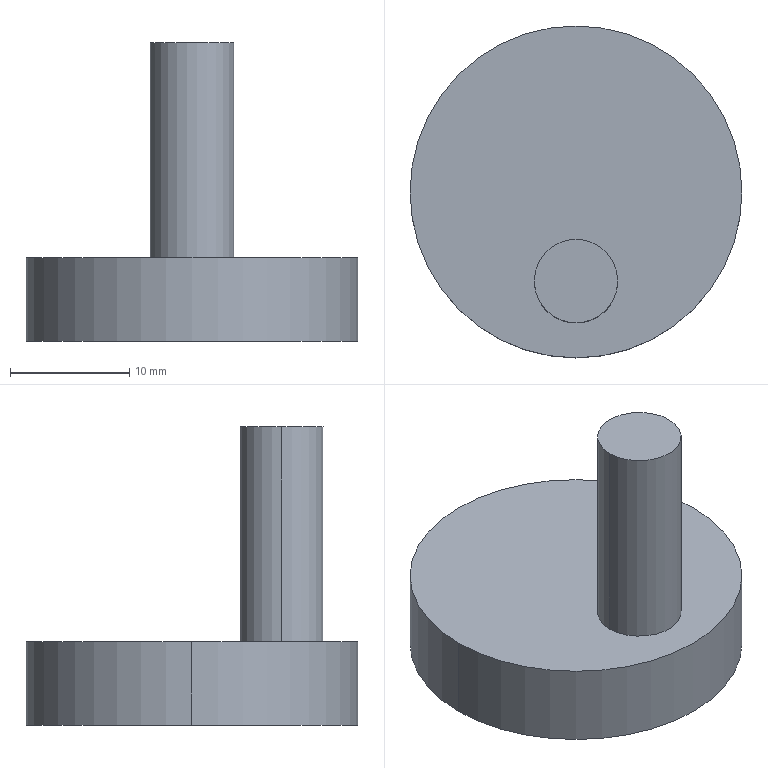Part | SolidWorks | features Cut 1, Extrusion 1, ICE 1 | 1 solid | 10 faces | box 27.8 x 27.8 x 25 mm | volume 4655 mm3 | cylinder 6 | plane 4 | commonest cylinder face diameters 7 x2 7.8 x2 27.8 x2
STEP:
#1=CARTESIAN_POINT('',(4.113,-42.5,20.));
#2=VERTEX_POINT('',#1);
#3=CARTESIAN_POINT('',(-2.887,-42.5,20.));
#4=VERTEX_POINT('',#3);
#5=CARTESIAN_POINT('',(0.6135,-42.5,20.));
#6=DIRECTION('',(0.,0.,1.));
#7=DIRECTION('',(1.,0.,0.));
#8=AXIS2_PLACEMENT_3D('',#5,#6,#7);
#9=CIRCLE('',#8,3.5);
#10=EDGE_CURVE('',#2,#4,#9,.T.);
#11=ORIENTED_EDGE('',*,*,#10,.F.);
#12=CARTESIAN_POINT('',(4.113,-42.5,2.));
#13=VERTEX_POINT('',#12);
#14=CARTESIAN_POINT('',(4.113,-42.5,20.));
#15=DIRECTION('',(0.,0.,-1.));
#16=VECTOR('',#15,1000.);
#17=LINE('',#14,#16);
#18=EDGE_CURVE('',#2,#13,#17,.T.);
#19=ORIENTED_EDGE('',*,*,#18,.T.);
#20=CARTESIAN_POINT('',(-2.887,-42.5,2.));
#21=VERTEX_POINT('',#20);
#22=CARTESIAN_POINT('',(0.6135,-42.5,2.));
#23=DIRECTION('',(0.,0.,1.));
#24=DIRECTION('',(1.,0.,0.));
#25=AXIS2_PLACEMENT_3D('',#22,#23,#24);
#26=CIRCLE('',#25,3.5);
#27=EDGE_CURVE('',#13,#21,#26,.T.);
#28=ORIENTED_EDGE('',*,*,#27,.T.);
#29=CARTESIAN_POINT('',(-2.887,-42.5,20.));
#30=DIRECTION('',(0.,0.,-1.));
#31=VECTOR('',#30,1000.);
#32=LINE('',#29,#31);
#33=EDGE_CURVE('',#4,#21,#32,.T.);
#34=ORIENTED_EDGE('',*,*,#33,.F.);
#35=EDGE_LOOP('',(#11,#19,#28,#34));
#36=FACE_OUTER_BOUND('',#35,.T.);
#37=CARTESIAN_POINT('',(0.6135,-42.5,20.));
#38=DIRECTION('',(0.,0.,-1.));
#39=DIRECTION('',(-1.,0.,0.));
#40=AXIS2_PLACEMENT_3D('',#37,#38,#39);
#41=CYLINDRICAL_SURFACE('',#40,3.5);
#42=ADVANCED_FACE('',(#36),#41,.T.);
#43=CARTESIAN_POINT('',(4.513,-35.,1.));
#44=VERTEX_POINT('',#43);
#45=CARTESIAN_POINT('',(-3.287,-35.,1.));
#46=VERTEX_POINT('',#45);
#47=CARTESIAN_POINT('',(0.6135,-35.,1.));
#48=DIRECTION('',(0.,0.,-1.));
#49=DIRECTION('',(-1.,0.,0.));
#50=AXIS2_PLACEMENT_3D('',#47,#48,#49);
#51=CIRCLE('',#50,3.9);
#52=EDGE_CURVE('',#44,#46,#51,.T.);
#53=ORIENTED_EDGE('',*,*,#52,.F.);
#54=CARTESIAN_POINT('',(4.513,-35.,-5.));
#55=VERTEX_POINT('',#54);
#56=CARTESIAN_POINT('',(4.513,-35.,1.));
#57=DIRECTION('',(0.,0.,-1.));
#58=VECTOR('',#57,1000.);
#59=LINE('',#56,#58);
#60=EDGE_CURVE('',#44,#55,#59,.T.);
#61=ORIENTED_EDGE('',*,*,#60,.T.);
#62=CARTESIAN_POINT('',(-3.287,-35.,-5.));
#63=VERTEX_POINT('',#62);
#64=CARTESIAN_POINT('',(0.6135,-35.,-5.));
#65=DIRECTION('',(0.,0.,-1.));
#66=DIRECTION('',(-1.,0.,0.));
#67=AXIS2_PLACEMENT_3D('',#64,#65,#66);
#68=CIRCLE('',#67,3.9);
#69=EDGE_CURVE('',#55,#63,#68,.T.);
#70=ORIENTED_EDGE('',*,*,#69,.T.);
#71=CARTESIAN_POINT('',(-3.287,-35.,1.));
#72=DIRECTION('',(0.,0.,-1.));
#73=VECTOR('',#72,1000.);
#74=LINE('',#71,#73);
#75=EDGE_CURVE('',#46,#63,#74,.T.);
#76=ORIENTED_EDGE('',*,*,#75,.F.);
#77=EDGE_LOOP('',(#53,#61,#70,#76));
#78=FACE_OUTER_BOUND('',#77,.T.);
#79=CARTESIAN_POINT('',(0.6135,-35.,1.));
#80=DIRECTION('',(0.,0.,-1.));
#81=DIRECTION('',(-1.,0.,0.));
#82=AXIS2_PLACEMENT_3D('',#79,#80,#81);
#83=CYLINDRICAL_SURFACE('',#82,3.9);
#84=ADVANCED_FACE('',(#78),#83,.F.);
#85=CARTESIAN_POINT('',(14.513,-35.,2.));
#86=VERTEX_POINT('',#85);
#87=CARTESIAN_POINT('',(-13.287,-35.,2.));
#88=VERTEX_POINT('',#87);
#89=CARTESIAN_POINT('',(0.6135,-35.,2.));
#90=DIRECTION('',(0.,0.,1.));
#91=DIRECTION('',(1.,0.,0.));
#92=AXIS2_PLACEMENT_3D('',#89,#90,#91);
#93=CIRCLE('',#92,13.9);
#94=EDGE_CURVE('',#86,#88,#93,.T.);
#95=ORIENTED_EDGE('',*,*,#94,.F.);
#96=CARTESIAN_POINT('',(14.513,-35.,-5.));
#97=VERTEX_POINT('',#96);
#98=CARTESIAN_POINT('',(14.513,-35.,2.));
#99=DIRECTION('',(0.,0.,-1.));
#100=VECTOR('',#99,1000.);
#101=LINE('',#98,#100);
#102=EDGE_CURVE('',#86,#97,#101,.T.);
#103=ORIENTED_EDGE('',*,*,#102,.T.);
#104=CARTESIAN_POINT('',(-13.287,-35.,-5.));
#105=VERTEX_POINT('',#104);
#106=CARTESIAN_POINT('',(0.6135,-35.,-5.));
#107=DIRECTION('',(0.,0.,1.));
#108=DIRECTION('',(1.,0.,0.));
#109=AXIS2_PLACEMENT_3D('',#106,#107,#108);
#110=CIRCLE('',#109,13.9);
#111=EDGE_CURVE('',#97,#105,#110,.T.);
#112=ORIENTED_EDGE('',*,*,#111,.T.);
#113=CARTESIAN_POINT('',(-13.287,-35.,2.));
#114=DIRECTION('',(0.,0.,-1.));
#115=VECTOR('',#114,1000.);
#116=LINE('',#113,#115);
#117=EDGE_CURVE('',#88,#105,#116,.T.);
#118=ORIENTED_EDGE('',*,*,#117,.F.);
#119=EDGE_LOOP('',(#95,#103,#112,#118));
#120=FACE_OUTER_BOUND('',#119,.T.);
#121=CARTESIAN_POINT('',(0.6135,-35.,2.));
#122=DIRECTION('',(0.,0.,-1.));
#123=DIRECTION('',(-1.,0.,0.));
#124=AXIS2_PLACEMENT_3D('',#121,#122,#123);
#125=CYLINDRICAL_SURFACE('',#124,13.9);
#126=ADVANCED_FACE('',(#120),#125,.T.);
#127=ORIENTED_EDGE('',*,*,#102,.F.);
#128=CARTESIAN_POINT('',(0.6135,-35.,2.));
#129=DIRECTION('',(0.,0.,1.));
#130=DIRECTION('',(1.,0.,0.));
#131=AXIS2_PLACEMENT_3D('',#128,#129,#130);
#132=CIRCLE('',#131,13.9);
#133=EDGE_CURVE('',#88,#86,#132,.T.);
#134=ORIENTED_EDGE('',*,*,#133,.F.);
#135=ORIENTED_EDGE('',*,*,#117,.T.);
#136=CARTESIAN_POINT('',(0.6135,-35.,-5.));
#137=DIRECTION('',(0.,0.,1.));
#138=DIRECTION('',(1.,0.,0.));
#139=AXIS2_PLACEMENT_3D('',#136,#137,#138);
#140=CIRCLE('',#139,13.9);
#141=EDGE_CURVE('',#105,#97,#140,.T.);
#142=ORIENTED_EDGE('',*,*,#141,.T.);
#143=EDGE_LOOP('',(#127,#134,#135,#142));
#144=FACE_OUTER_BOUND('',#143,.T.);
#145=CARTESIAN_POINT('',(0.6135,-35.,2.));
#146=DIRECTION('',(0.,0.,-1.));
#147=DIRECTION('',(-1.,0.,0.));
#148=AXIS2_PLACEMENT_3D('',#145,#146,#147);
#149=CYLINDRICAL_SURFACE('',#148,13.9);
#150=ADVANCED_FACE('',(#144),#149,.T.);
#151=CARTESIAN_POINT('',(0.6135,-42.5,2.));
#152=DIRECTION('',(0.,0.,1.));
#153=DIRECTION('',(1.,0.,0.));
#154=AXIS2_PLACEMENT_3D('',#151,#152,#153);
#155=CIRCLE('',#154,3.5);
#156=EDGE_CURVE('',#21,#13,#155,.T.);
#157=ORIENTED_EDGE('',*,*,#156,.F.);
#158=ORIENTED_EDGE('',*,*,#27,.F.);
#159=EDGE_LOOP('',(#157,#158));
#160=FACE_BOUND('',#159,.T.);
#161=ORIENTED_EDGE('',*,*,#133,.T.);
#162=ORIENTED_EDGE('',*,*,#94,.T.);
#163=EDGE_LOOP('',(#161,#162));
#164=FACE_OUTER_BOUND('',#163,.T.);
#165=CARTESIAN_POINT('',(0.6135,-35.,2.));
#166=DIRECTION('',(0.,0.,1.));
#167=DIRECTION('',(1.,0.,0.));
#168=AXIS2_PLACEMENT_3D('',#165,#166,#167);
#169=PLANE('',#168);
#170=ADVANCED_FACE('',(#160,#164),#169,.T.);
#171=CARTESIAN_POINT('',(0.6135,-35.,-5.));
#172=DIRECTION('',(0.,0.,-1.));
#173=DIRECTION('',(-1.,0.,0.));
#174=AXIS2_PLACEMENT_3D('',#171,#172,#173);
#175=CIRCLE('',#174,3.9);
#176=EDGE_CURVE('',#63,#55,#175,.T.);
#177=ORIENTED_EDGE('',*,*,#176,.F.);
#178=ORIENTED_EDGE('',*,*,#69,.F.);
#179=EDGE_LOOP('',(#177,#178));
#180=FACE_BOUND('',#179,.T.);
#181=ORIENTED_EDGE('',*,*,#141,.F.);
#182=ORIENTED_EDGE('',*,*,#111,.F.);
#183=EDGE_LOOP('',(#181,#182));
#184=FACE_OUTER_BOUND('',#183,.T.);
#185=CARTESIAN_POINT('',(0.6135,-35.,-5.));
#186=DIRECTION('',(0.,0.,1.));
#187=DIRECTION('',(1.,0.,0.));
#188=AXIS2_PLACEMENT_3D('',#185,#186,#187);
#189=PLANE('',#188);
#190=ADVANCED_FACE('',(#180,#184),#189,.F.);
#191=ORIENTED_EDGE('',*,*,#60,.F.);
#192=CARTESIAN_POINT('',(0.6135,-35.,1.));
#193=DIRECTION('',(0.,0.,-1.));
#194=DIRECTION('',(-1.,0.,0.));
#195=AXIS2_PLACEMENT_3D('',#192,#193,#194);
#196=CIRCLE('',#195,3.9);
#197=EDGE_CURVE('',#46,#44,#196,.T.);
#198=ORIENTED_EDGE('',*,*,#197,.F.);
#199=ORIENTED_EDGE('',*,*,#75,.T.);
#200=ORIENTED_EDGE('',*,*,#176,.T.);
#201=EDGE_LOOP('',(#191,#198,#199,#200));
#202=FACE_OUTER_BOUND('',#201,.T.);
#203=CARTESIAN_POINT('',(0.6135,-35.,1.));
#204=DIRECTION('',(0.,0.,-1.));
#205=DIRECTION('',(-1.,0.,0.));
#206=AXIS2_PLACEMENT_3D('',#203,#204,#205);
#207=CYLINDRICAL_SURFACE('',#206,3.9);
#208=ADVANCED_FACE('',(#202),#207,.F.);
#209=ORIENTED_EDGE('',*,*,#197,.T.);
#210=ORIENTED_EDGE('',*,*,#52,.T.);
#211=EDGE_LOOP('',(#209,#210));
#212=FACE_OUTER_BOUND('',#211,.T.);
#213=CARTESIAN_POINT('',(0.6135,-35.,1.));
#214=DIRECTION('',(0.,0.,-1.));
#215=DIRECTION('',(-1.,0.,0.));
#216=AXIS2_PLACEMENT_3D('',#213,#214,#215);
#217=PLANE('',#216);
#218=ADVANCED_FACE('',(#212),#217,.T.);
#219=ORIENTED_EDGE('',*,*,#18,.F.);
#220=CARTESIAN_POINT('',(0.6135,-42.5,20.));
#221=DIRECTION('',(0.,0.,1.));
#222=DIRECTION('',(1.,0.,0.));
#223=AXIS2_PLACEMENT_3D('',#220,#221,#222);
#224=CIRCLE('',#223,3.5);
#225=EDGE_CURVE('',#4,#2,#224,.T.);
#226=ORIENTED_EDGE('',*,*,#225,.F.);
#227=ORIENTED_EDGE('',*,*,#33,.T.);
#228=ORIENTED_EDGE('',*,*,#156,.T.);
#229=EDGE_LOOP('',(#219,#226,#227,#228));
#230=FACE_OUTER_BOUND('',#229,.T.);
#231=CARTESIAN_POINT('',(0.6135,-42.5,20.));
#232=DIRECTION('',(0.,0.,-1.));
#233=DIRECTION('',(-1.,0.,0.));
#234=AXIS2_PLACEMENT_3D('',#231,#232,#233);
#235=CYLINDRICAL_SURFACE('',#234,3.5);
#236=ADVANCED_FACE('',(#230),#235,.T.);
#237=ORIENTED_EDGE('',*,*,#225,.T.);
#238=ORIENTED_EDGE('',*,*,#10,.T.);
#239=EDGE_LOOP('',(#237,#238));
#240=FACE_OUTER_BOUND('',#239,.T.);
#241=CARTESIAN_POINT('',(0.6135,-42.5,20.));
#242=DIRECTION('',(0.,0.,1.));
#243=DIRECTION('',(1.,0.,0.));
#244=AXIS2_PLACEMENT_3D('',#241,#242,#243);
#245=PLANE('',#244);
#246=ADVANCED_FACE('',(#240),#245,.T.);
#247=CLOSED_SHELL('',(#42,#84,#126,#150,#170,#190,#208,#218,#236,#246));
#248=MANIFOLD_SOLID_BREP('',#247);
#249=CARTESIAN_POINT('',(0.,0.,0.));
#250=DIRECTION('',(0.,0.,1.));
#251=DIRECTION('',(1.,0.,0.));
#252=AXIS2_PLACEMENT_3D('',#249,#250,#251);
#253=(LENGTH_UNIT()NAMED_UNIT(*)SI_UNIT(.MILLI.,.METRE.));
#254=UNCERTAINTY_MEASURE_WITH_UNIT(LENGTH_MEASURE(0.00001),#253,'','');
#255=(NAMED_UNIT(*)PLANE_ANGLE_UNIT()SI_UNIT($,.RADIAN.));
#256=(NAMED_UNIT(*)SI_UNIT($,.STERADIAN.)SOLID_ANGLE_UNIT());
#257=(GEOMETRIC_REPRESENTATION_CONTEXT(3)GLOBAL_UNCERTAINTY_ASSIGNED_CONTEXT((#254))GLOBAL_UNIT_ASSIGNED_CONTEXT((#253,#255,#256))REPRESENTATION_CONTEXT('',''));
#258=ADVANCED_BREP_SHAPE_REPRESENTATION('',(#248,#252),#257);